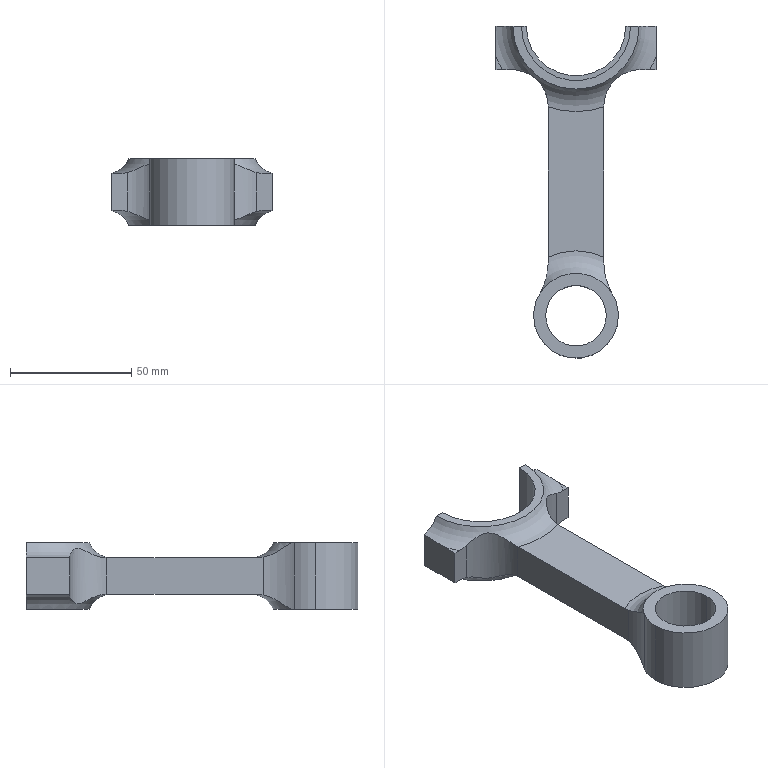Part | SolidWorks | features Fillet 4, ICE 3, Extrusion 1, MirrorPattern 1 | 1 solid | 34 faces | box 66 x 137 x 27.5 mm | volume 56707 mm3 | plane 19 | cylinder 11 | torus 4 | commonest cylinder face diameters 35 x3 25 x2 30 x2 50 x2 41 x1 45 x1
STEP:
#1=CARTESIAN_POINT('',(-12.5,-110.5,13.75));
#2=VERTEX_POINT('',#1);
#3=CARTESIAN_POINT('',(12.5,-110.5,13.75));
#4=VERTEX_POINT('',#3);
#5=CARTESIAN_POINT('',(0.,-110.5,13.75));
#6=DIRECTION('',(0.,0.,1.));
#7=DIRECTION('',(1.,0.,0.));
#8=AXIS2_PLACEMENT_3D('',#5,#6,#7);
#9=CIRCLE('',#8,12.5);
#10=EDGE_CURVE('',#2,#4,#9,.T.);
#11=ORIENTED_EDGE('',*,*,#10,.T.);
#12=CARTESIAN_POINT('',(12.5,-110.5,-13.75));
#13=VERTEX_POINT('',#12);
#14=CARTESIAN_POINT('',(12.5,-110.5,13.75));
#15=DIRECTION('',(0.,0.,-1.));
#16=VECTOR('',#15,1000.);
#17=LINE('',#14,#16);
#18=EDGE_CURVE('',#4,#13,#17,.T.);
#19=ORIENTED_EDGE('',*,*,#18,.T.);
#20=CARTESIAN_POINT('',(-12.5,-110.5,-13.75));
#21=VERTEX_POINT('',#20);
#22=CARTESIAN_POINT('',(0.,-110.5,-13.75));
#23=DIRECTION('',(0.,0.,1.));
#24=DIRECTION('',(1.,0.,0.));
#25=AXIS2_PLACEMENT_3D('',#22,#23,#24);
#26=CIRCLE('',#25,12.5);
#27=EDGE_CURVE('',#21,#13,#26,.T.);
#28=ORIENTED_EDGE('',*,*,#27,.F.);
#29=CARTESIAN_POINT('',(-12.5,-110.5,13.75));
#30=DIRECTION('',(0.,0.,-1.));
#31=VECTOR('',#30,1000.);
#32=LINE('',#29,#31);
#33=EDGE_CURVE('',#2,#21,#32,.T.);
#34=ORIENTED_EDGE('',*,*,#33,.F.);
#35=EDGE_LOOP('',(#11,#19,#28,#34));
#36=FACE_OUTER_BOUND('',#35,.T.);
#37=CARTESIAN_POINT('',(0.,-110.5,13.75));
#38=DIRECTION('',(0.,0.,-1.));
#39=DIRECTION('',(-1.,0.,0.));
#40=AXIS2_PLACEMENT_3D('',#37,#38,#39);
#41=CYLINDRICAL_SURFACE('',#40,12.5);
#42=ADVANCED_FACE('',(#36),#41,.F.);
#43=CARTESIAN_POINT('',(17.5,-110.5,13.75));
#44=VERTEX_POINT('',#43);
#45=CARTESIAN_POINT('',(15.029,-101.535,13.75));
#46=VERTEX_POINT('',#45);
#47=CARTESIAN_POINT('',(0.,-110.5,13.75));
#48=DIRECTION('',(0.,0.,1.));
#49=DIRECTION('',(1.,0.,0.));
#50=AXIS2_PLACEMENT_3D('',#47,#48,#49);
#51=CIRCLE('',#50,17.5);
#52=EDGE_CURVE('',#44,#46,#51,.T.);
#53=ORIENTED_EDGE('',*,*,#52,.F.);
#54=CARTESIAN_POINT('',(17.5,-110.5,-13.75));
#55=VERTEX_POINT('',#54);
#56=CARTESIAN_POINT('',(17.5,-110.5,13.75));
#57=DIRECTION('',(0.,0.,-1.));
#58=VECTOR('',#57,1000.);
#59=LINE('',#56,#58);
#60=EDGE_CURVE('',#44,#55,#59,.T.);
#61=ORIENTED_EDGE('',*,*,#60,.T.);
#62=CARTESIAN_POINT('',(15.029,-101.535,-13.75));
#63=VERTEX_POINT('',#62);
#64=CARTESIAN_POINT('',(0.,-110.5,-13.75));
#65=DIRECTION('',(0.,0.,1.));
#66=DIRECTION('',(1.,0.,0.));
#67=AXIS2_PLACEMENT_3D('',#64,#65,#66);
#68=CIRCLE('',#67,17.5);
#69=EDGE_CURVE('',#55,#63,#68,.T.);
#70=ORIENTED_EDGE('',*,*,#69,.T.);
#71=CARTESIAN_POINT('',(15.029,-101.535,13.75));
#72=DIRECTION('',(0.,0.,1.));
#73=VECTOR('',#72,1000.);
#74=LINE('',#71,#73);
#75=EDGE_CURVE('',#63,#46,#74,.T.);
#76=ORIENTED_EDGE('',*,*,#75,.T.);
#77=EDGE_LOOP('',(#53,#61,#70,#76));
#78=FACE_OUTER_BOUND('',#77,.T.);
#79=CARTESIAN_POINT('',(0.,-110.5,13.75));
#80=DIRECTION('',(0.,0.,-1.));
#81=DIRECTION('',(-1.,0.,0.));
#82=AXIS2_PLACEMENT_3D('',#79,#80,#81);
#83=CYLINDRICAL_SURFACE('',#82,17.5);
#84=ADVANCED_FACE('',(#78),#83,.T.);
#85=ORIENTED_EDGE('',*,*,#60,.F.);
#86=CARTESIAN_POINT('',(-17.5,-110.5,13.75));
#87=VERTEX_POINT('',#86);
#88=CARTESIAN_POINT('',(0.,-110.5,13.75));
#89=DIRECTION('',(0.,0.,1.));
#90=DIRECTION('',(1.,0.,0.));
#91=AXIS2_PLACEMENT_3D('',#88,#89,#90);
#92=CIRCLE('',#91,17.5);
#93=EDGE_CURVE('',#87,#44,#92,.T.);
#94=ORIENTED_EDGE('',*,*,#93,.F.);
#95=CARTESIAN_POINT('',(-17.5,-110.5,-13.75));
#96=VERTEX_POINT('',#95);
#97=CARTESIAN_POINT('',(-17.5,-110.5,13.75));
#98=DIRECTION('',(0.,0.,-1.));
#99=VECTOR('',#98,1000.);
#100=LINE('',#97,#99);
#101=EDGE_CURVE('',#87,#96,#100,.T.);
#102=ORIENTED_EDGE('',*,*,#101,.T.);
#103=CARTESIAN_POINT('',(0.,-110.5,-13.75));
#104=DIRECTION('',(0.,0.,1.));
#105=DIRECTION('',(1.,0.,0.));
#106=AXIS2_PLACEMENT_3D('',#103,#104,#105);
#107=CIRCLE('',#106,17.5);
#108=EDGE_CURVE('',#96,#55,#107,.T.);
#109=ORIENTED_EDGE('',*,*,#108,.T.);
#110=EDGE_LOOP('',(#85,#94,#102,#109));
#111=FACE_OUTER_BOUND('',#110,.T.);
#112=CARTESIAN_POINT('',(0.,-110.5,13.75));
#113=DIRECTION('',(0.,0.,-1.));
#114=DIRECTION('',(-1.,0.,0.));
#115=AXIS2_PLACEMENT_3D('',#112,#113,#114);
#116=CYLINDRICAL_SURFACE('',#115,17.5);
#117=ADVANCED_FACE('',(#111),#116,.T.);
#118=CARTESIAN_POINT('',(26.,9.,-13.75));
#119=VERTEX_POINT('',#118);
#120=CARTESIAN_POINT('',(20.5,9.,-13.75));
#121=VERTEX_POINT('',#120);
#122=CARTESIAN_POINT('',(33.,9.,-13.75));
#123=DIRECTION('',(-1.,0.,0.));
#124=VECTOR('',#123,1000.);
#125=LINE('',#122,#124);
#126=EDGE_CURVE('',#119,#121,#125,.T.);
#127=ORIENTED_EDGE('',*,*,#126,.T.);
#128=CARTESIAN_POINT('',(20.5,9.,-12.75));
#129=VERTEX_POINT('',#128);
#130=CARTESIAN_POINT('',(20.5,9.,-14.97));
#131=DIRECTION('',(0.,0.,1.));
#132=VECTOR('',#131,1000.);
#133=LINE('',#130,#132);
#134=EDGE_CURVE('',#121,#129,#133,.T.);
#135=ORIENTED_EDGE('',*,*,#134,.T.);
#136=CARTESIAN_POINT('',(22.5,9.,-12.75));
#137=VERTEX_POINT('',#136);
#138=CARTESIAN_POINT('',(33.,9.,-12.75));
#139=DIRECTION('',(-1.,0.,0.));
#140=VECTOR('',#139,1000.);
#141=LINE('',#138,#140);
#142=EDGE_CURVE('',#137,#129,#141,.T.);
#143=ORIENTED_EDGE('',*,*,#142,.F.);
#144=CARTESIAN_POINT('',(22.5,9.,13.75));
#145=VERTEX_POINT('',#144);
#146=CARTESIAN_POINT('',(22.5,9.,-12.75));
#147=DIRECTION('',(0.,0.,1.));
#148=VECTOR('',#147,1000.);
#149=LINE('',#146,#148);
#150=EDGE_CURVE('',#137,#145,#149,.T.);
#151=ORIENTED_EDGE('',*,*,#150,.T.);
#152=CARTESIAN_POINT('',(26.,9.,13.75));
#153=VERTEX_POINT('',#152);
#154=CARTESIAN_POINT('',(33.,9.,13.75));
#155=DIRECTION('',(-1.,0.,0.));
#156=VECTOR('',#155,1000.);
#157=LINE('',#154,#156);
#158=EDGE_CURVE('',#153,#145,#157,.T.);
#159=ORIENTED_EDGE('',*,*,#158,.F.);
#160=CARTESIAN_POINT('',(33.,9.,7.761));
#161=VERTEX_POINT('',#160);
#162=CARTESIAN_POINT('',(35.27,9.,17.5));
#163=DIRECTION('',(0.,-1.,0.));
#164=DIRECTION('',(1.,0.,0.));
#165=AXIS2_PLACEMENT_3D('',#162,#163,#164);
#166=CIRCLE('',#165,10.);
#167=EDGE_CURVE('',#153,#161,#166,.T.);
#168=ORIENTED_EDGE('',*,*,#167,.T.);
#169=CARTESIAN_POINT('',(33.,9.,-7.761));
#170=VERTEX_POINT('',#169);
#171=CARTESIAN_POINT('',(33.,9.,13.75));
#172=DIRECTION('',(0.,0.,-1.));
#173=VECTOR('',#172,1000.);
#174=LINE('',#171,#173);
#175=EDGE_CURVE('',#161,#170,#174,.T.);
#176=ORIENTED_EDGE('',*,*,#175,.T.);
#177=CARTESIAN_POINT('',(35.27,9.,-17.5));
#178=DIRECTION('',(0.,-1.,0.));
#179=DIRECTION('',(1.,0.,0.));
#180=AXIS2_PLACEMENT_3D('',#177,#178,#179);
#181=CIRCLE('',#180,10.);
#182=EDGE_CURVE('',#170,#119,#181,.T.);
#183=ORIENTED_EDGE('',*,*,#182,.T.);
#184=EDGE_LOOP('',(#127,#135,#143,#151,#159,#168,#176,#183));
#185=FACE_OUTER_BOUND('',#184,.T.);
#186=CARTESIAN_POINT('',(33.,9.,13.75));
#187=DIRECTION('',(0.,-1.,0.));
#188=DIRECTION('',(1.,0.,0.));
#189=AXIS2_PLACEMENT_3D('',#186,#187,#188);
#190=PLANE('',#189);
#191=ADVANCED_FACE('',(#185),#190,.F.);
#192=CARTESIAN_POINT('',(-33.,-3.45,-7.5));
#193=VERTEX_POINT('',#192);
#194=CARTESIAN_POINT('',(-33.,-9.,-7.5));
#195=VERTEX_POINT('',#194);
#196=CARTESIAN_POINT('',(-33.,0.,-7.5));
#197=DIRECTION('',(0.,-1.,0.));
#198=VECTOR('',#197,1000.);
#199=LINE('',#196,#198);
#200=EDGE_CURVE('',#193,#195,#199,.T.);
#201=ORIENTED_EDGE('',*,*,#200,.F.);
#202=CARTESIAN_POINT('',(-30.331,-9.,-7.5));
#203=VERTEX_POINT('',#202);
#204=CARTESIAN_POINT('',(0.,9.,-7.5));
#205=DIRECTION('',(0.,0.,1.));
#206=DIRECTION('',(-1.,0.,0.));
#207=AXIS2_PLACEMENT_3D('',#204,#205,#206);
#208=CIRCLE('',#207,35.27);
#209=EDGE_CURVE('',#193,#203,#208,.T.);
#210=ORIENTED_EDGE('',*,*,#209,.T.);
#211=CARTESIAN_POINT('',(0.,-9.,-7.5));
#212=DIRECTION('',(1.,0.,0.));
#213=VECTOR('',#212,1000.);
#214=LINE('',#211,#213);
#215=EDGE_CURVE('',#195,#203,#214,.T.);
#216=ORIENTED_EDGE('',*,*,#215,.F.);
#217=EDGE_LOOP('',(#201,#210,#216));
#218=FACE_OUTER_BOUND('',#217,.T.);
#219=CARTESIAN_POINT('',(0.,0.,-7.5));
#220=DIRECTION('',(0.,0.,-1.));
#221=DIRECTION('',(1.,0.,0.));
#222=AXIS2_PLACEMENT_3D('',#219,#220,#221);
#223=PLANE('',#222);
#224=ADVANCED_FACE('',(#218),#223,.T.);
#225=CARTESIAN_POINT('',(11.5,-86.326,-7.5));
#226=VERTEX_POINT('',#225);
#227=CARTESIAN_POINT('',(11.5,-24.343,-7.5));
#228=VERTEX_POINT('',#227);
#229=CARTESIAN_POINT('',(11.5,0.,-7.5));
#230=DIRECTION('',(0.,1.,0.));
#231=VECTOR('',#230,1000.);
#232=LINE('',#229,#231);
#233=EDGE_CURVE('',#226,#228,#232,.T.);
#234=ORIENTED_EDGE('',*,*,#233,.F.);
#235=CARTESIAN_POINT('',(-11.5,-86.326,-7.5));
#236=VERTEX_POINT('',#235);
#237=CARTESIAN_POINT('',(0.,-110.5,-7.5));
#238=DIRECTION('',(0.,0.,1.));
#239=DIRECTION('',(-1.,0.,0.));
#240=AXIS2_PLACEMENT_3D('',#237,#238,#239);
#241=CIRCLE('',#240,26.77);
#242=EDGE_CURVE('',#226,#236,#241,.T.);
#243=ORIENTED_EDGE('',*,*,#242,.T.);
#244=CARTESIAN_POINT('',(-11.5,-24.343,-7.5));
#245=VERTEX_POINT('',#244);
#246=CARTESIAN_POINT('',(-11.5,0.,-7.5));
#247=DIRECTION('',(0.,-1.,0.));
#248=VECTOR('',#247,1000.);
#249=LINE('',#246,#248);
#250=EDGE_CURVE('',#245,#236,#249,.T.);
#251=ORIENTED_EDGE('',*,*,#250,.F.);
#252=CARTESIAN_POINT('',(0.,9.,-7.5));
#253=DIRECTION('',(0.,0.,1.));
#254=DIRECTION('',(-1.,0.,0.));
#255=AXIS2_PLACEMENT_3D('',#252,#253,#254);
#256=CIRCLE('',#255,35.27);
#257=EDGE_CURVE('',#245,#228,#256,.T.);
#258=ORIENTED_EDGE('',*,*,#257,.T.);
#259=EDGE_LOOP('',(#234,#243,#251,#258));
#260=FACE_OUTER_BOUND('',#259,.T.);
#261=CARTESIAN_POINT('',(0.,0.,-7.5));
#262=DIRECTION('',(0.,0.,-1.));
#263=DIRECTION('',(1.,0.,0.));
#264=AXIS2_PLACEMENT_3D('',#261,#262,#263);
#265=PLANE('',#264);
#266=ADVANCED_FACE('',(#260),#265,.T.);
#267=CARTESIAN_POINT('',(33.,-9.,7.5));
#268=VERTEX_POINT('',#267);
#269=CARTESIAN_POINT('',(33.,-3.45,7.5));
#270=VERTEX_POINT('',#269);
#271=CARTESIAN_POINT('',(33.,0.,7.5));
#272=DIRECTION('',(0.,1.,0.));
#273=VECTOR('',#272,1000.);
#274=LINE('',#271,#273);
#275=EDGE_CURVE('',#268,#270,#274,.T.);
#276=ORIENTED_EDGE('',*,*,#275,.T.);
#277=CARTESIAN_POINT('',(30.331,-9.,7.5));
#278=VERTEX_POINT('',#277);
#279=CARTESIAN_POINT('',(0.,9.,7.5));
#280=DIRECTION('',(0.,0.,-1.));
#281=DIRECTION('',(1.,0.,0.));
#282=AXIS2_PLACEMENT_3D('',#279,#280,#281);
#283=CIRCLE('',#282,35.27);
#284=EDGE_CURVE('',#270,#278,#283,.T.);
#285=ORIENTED_EDGE('',*,*,#284,.T.);
#286=CARTESIAN_POINT('',(0.,-9.,7.5));
#287=DIRECTION('',(1.,0.,0.));
#288=VECTOR('',#287,1000.);
#289=LINE('',#286,#288);
#290=EDGE_CURVE('',#278,#268,#289,.T.);
#291=ORIENTED_EDGE('',*,*,#290,.T.);
#292=EDGE_LOOP('',(#276,#285,#291));
#293=FACE_OUTER_BOUND('',#292,.T.);
#294=CARTESIAN_POINT('',(0.,0.,7.5));
#295=DIRECTION('',(0.,0.,1.));
#296=DIRECTION('',(1.,0.,0.));
#297=AXIS2_PLACEMENT_3D('',#294,#295,#296);
#298=PLANE('',#297);
#299=ADVANCED_FACE('',(#293),#298,.T.);
#300=CARTESIAN_POINT('',(-11.5,-24.343,7.5));
#301=VERTEX_POINT('',#300);
#302=CARTESIAN_POINT('',(-11.5,-86.326,7.5));
#303=VERTEX_POINT('',#302);
#304=CARTESIAN_POINT('',(-11.5,0.,7.5));
#305=DIRECTION('',(0.,-1.,0.));
#306=VECTOR('',#305,1000.);
#307=LINE('',#304,#306);
#308=EDGE_CURVE('',#301,#303,#307,.T.);
#309=ORIENTED_EDGE('',*,*,#308,.T.);
#310=CARTESIAN_POINT('',(11.5,-86.326,7.5));
#311=VERTEX_POINT('',#310);
#312=CARTESIAN_POINT('',(0.,-110.5,7.5));
#313=DIRECTION('',(0.,0.,-1.));
#314=DIRECTION('',(1.,0.,0.));
#315=AXIS2_PLACEMENT_3D('',#312,#313,#314);
#316=CIRCLE('',#315,26.77);
#317=EDGE_CURVE('',#303,#311,#316,.T.);
#318=ORIENTED_EDGE('',*,*,#317,.T.);
#319=CARTESIAN_POINT('',(11.5,-24.343,7.5));
#320=VERTEX_POINT('',#319);
#321=CARTESIAN_POINT('',(11.5,0.,7.5));
#322=DIRECTION('',(0.,1.,0.));
#323=VECTOR('',#322,1000.);
#324=LINE('',#321,#323);
#325=EDGE_CURVE('',#311,#320,#324,.T.);
#326=ORIENTED_EDGE('',*,*,#325,.T.);
#327=CARTESIAN_POINT('',(0.,9.,7.5));
#328=DIRECTION('',(0.,0.,-1.));
#329=DIRECTION('',(1.,0.,0.));
#330=AXIS2_PLACEMENT_3D('',#327,#328,#329);
#331=CIRCLE('',#330,35.27);
#332=EDGE_CURVE('',#320,#301,#331,.T.);
#333=ORIENTED_EDGE('',*,*,#332,.T.);
#334=EDGE_LOOP('',(#309,#318,#326,#333));
#335=FACE_OUTER_BOUND('',#334,.T.);
#336=CARTESIAN_POINT('',(0.,0.,7.5));
#337=DIRECTION('',(0.,0.,1.));
#338=DIRECTION('',(1.,0.,0.));
#339=AXIS2_PLACEMENT_3D('',#336,#337,#338);
#340=PLANE('',#339);
#341=ADVANCED_FACE('',(#335),#340,.T.);
#342=CARTESIAN_POINT('',(-33.,9.,7.761));
#343=VERTEX_POINT('',#342);
#344=CARTESIAN_POINT('',(-33.,9.,-7.761));
#345=VERTEX_POINT('',#344);
#346=CARTESIAN_POINT('',(-33.,9.,13.75));
#347=DIRECTION('',(0.,0.,-1.));
#348=VECTOR('',#347,1000.);
#349=LINE('',#346,#348);
#350=EDGE_CURVE('',#343,#345,#349,.T.);
#351=ORIENTED_EDGE('',*,*,#350,.T.);
#352=CARTESIAN_POINT('',(-33.,9.,-7.761));
#353=CARTESIAN_POINT('',(-33.,7.962,-7.761));
#354=CARTESIAN_POINT('',(-33.,6.925,-7.749));
#355=CARTESIAN_POINT('',(-33.,4.85,-7.707));
#356=CARTESIAN_POINT('',(-33.,3.812,-7.676));
#357=CARTESIAN_POINT('',(-33.,0.7007,-7.578));
#358=CARTESIAN_POINT('',(-33.,-1.373,-7.5));
#359=CARTESIAN_POINT('',(-33.,-3.45,-7.5));
#360=B_SPLINE_CURVE_WITH_KNOTS('',3,(#352,#353,#354,#355,#356,#357,#358,#359),.UNSPECIFIED.,.F.,.F.,(4,2,2,4),(0.,0.003113,0.006226,0.01245),.UNSPECIFIED.);
#361=EDGE_CURVE('',#345,#193,#360,.T.);
#362=ORIENTED_EDGE('',*,*,#361,.T.);
#363=ORIENTED_EDGE('',*,*,#200,.T.);
#364=CARTESIAN_POINT('',(-33.,-9.,7.5));
#365=VERTEX_POINT('',#364);
#366=CARTESIAN_POINT('',(-33.,-9.,13.75));
#367=DIRECTION('',(0.,0.,-1.));
#368=VECTOR('',#367,1000.);
#369=LINE('',#366,#368);
#370=EDGE_CURVE('',#365,#195,#369,.T.);
#371=ORIENTED_EDGE('',*,*,#370,.F.);
#372=CARTESIAN_POINT('',(-33.,-3.45,7.5));
#373=VERTEX_POINT('',#372);
#374=CARTESIAN_POINT('',(-33.,0.,7.5));
#375=DIRECTION('',(0.,-1.,0.));
#376=VECTOR('',#375,1000.);
#377=LINE('',#374,#376);
#378=EDGE_CURVE('',#373,#365,#377,.T.);
#379=ORIENTED_EDGE('',*,*,#378,.F.);
#380=CARTESIAN_POINT('',(-33.,-3.45,7.5));
#381=CARTESIAN_POINT('',(-33.,-1.374,7.5));
#382=CARTESIAN_POINT('',(-33.,0.7005,7.578));
#383=CARTESIAN_POINT('',(-33.,3.812,7.676));
#384=CARTESIAN_POINT('',(-33.,4.849,7.707));
#385=CARTESIAN_POINT('',(-33.,6.924,7.749));
#386=CARTESIAN_POINT('',(-33.,7.962,7.761));
#387=CARTESIAN_POINT('',(-33.,9.,7.761));
#388=B_SPLINE_CURVE_WITH_KNOTS('',3,(#380,#381,#382,#383,#384,#385,#386,#387),.UNSPECIFIED.,.F.,.F.,(4,2,2,4),(0.,0.006226,0.009339,0.01245),.UNSPECIFIED.);
#389=EDGE_CURVE('',#373,#343,#388,.T.);
#390=ORIENTED_EDGE('',*,*,#389,.T.);
#391=EDGE_LOOP('',(#351,#362,#363,#371,#379,#390));
#392=FACE_OUTER_BOUND('',#391,.T.);
#393=CARTESIAN_POINT('',(-33.,-9.,13.75));
#394=DIRECTION('',(1.,0.,0.));
#395=DIRECTION('',(0.,0.,-1.));
#396=AXIS2_PLACEMENT_3D('',#393,#394,#395);
#397=PLANE('',#396);
#398=ADVANCED_FACE('',(#392),#397,.F.);
#399=ORIENTED_EDGE('',*,*,#215,.T.);
#400=CARTESIAN_POINT('',(-26.5,-9.,-8.038));
#401=VERTEX_POINT('',#400);
#402=CARTESIAN_POINT('',(-30.331,-9.,-7.5));
#403=CARTESIAN_POINT('',(-29.029,-9.,-7.5));
#404=CARTESIAN_POINT('',(-27.753,-9.,-7.684));
#405=CARTESIAN_POINT('',(-26.5,-9.,-8.038));
#406=B_SPLINE_CURVE_WITH_KNOTS('',3,(#402,#403,#404,#405),.UNSPECIFIED.,.F.,.F.,(4,4),(0.,0.003869),.UNSPECIFIED.);
#407=EDGE_CURVE('',#203,#401,#406,.T.);
#408=ORIENTED_EDGE('',*,*,#407,.T.);
#409=CARTESIAN_POINT('',(-26.5,-9.,8.038));
#410=VERTEX_POINT('',#409);
#411=CARTESIAN_POINT('',(-26.5,-9.,13.75));
#412=DIRECTION('',(0.,0.,1.));
#413=VECTOR('',#412,1000.);
#414=LINE('',#411,#413);
#415=EDGE_CURVE('',#401,#410,#414,.T.);
#416=ORIENTED_EDGE('',*,*,#415,.T.);
#417=CARTESIAN_POINT('',(-30.331,-9.,7.5));
#418=VERTEX_POINT('',#417);
#419=CARTESIAN_POINT('',(-26.5,-9.,8.038));
#420=CARTESIAN_POINT('',(-27.753,-9.,7.684));
#421=CARTESIAN_POINT('',(-29.029,-9.,7.5));
#422=CARTESIAN_POINT('',(-30.331,-9.,7.5));
#423=B_SPLINE_CURVE_WITH_KNOTS('',3,(#419,#420,#421,#422),.UNSPECIFIED.,.F.,.F.,(4,4),(0.,0.003869),.UNSPECIFIED.);
#424=EDGE_CURVE('',#410,#418,#423,.T.);
#425=ORIENTED_EDGE('',*,*,#424,.T.);
#426=CARTESIAN_POINT('',(0.,-9.,7.5));
#427=DIRECTION('',(1.,0.,0.));
#428=VECTOR('',#427,1000.);
#429=LINE('',#426,#428);
#430=EDGE_CURVE('',#365,#418,#429,.T.);
#431=ORIENTED_EDGE('',*,*,#430,.F.);
#432=ORIENTED_EDGE('',*,*,#370,.T.);
#433=EDGE_LOOP('',(#399,#408,#416,#425,#431,#432));
#434=FACE_OUTER_BOUND('',#433,.T.);
#435=CARTESIAN_POINT('',(-11.5,-9.,13.75));
#436=DIRECTION('',(0.,1.,0.));
#437=DIRECTION('',(-1.,0.,0.));
#438=AXIS2_PLACEMENT_3D('',#435,#436,#437);
#439=PLANE('',#438);
#440=ADVANCED_FACE('',(#434),#439,.F.);
#441=CARTESIAN_POINT('',(-11.5,-24.,7.505));
#442=VERTEX_POINT('',#441);
#443=CARTESIAN_POINT('',(-11.5,-24.,-7.505));
#444=VERTEX_POINT('',#443);
#445=CARTESIAN_POINT('',(-11.5,-24.,-13.75));
#446=DIRECTION('',(0.,0.,-1.));
#447=VECTOR('',#446,1000.);
#448=LINE('',#445,#447);
#449=EDGE_CURVE('',#442,#444,#448,.T.);
#450=ORIENTED_EDGE('',*,*,#449,.T.);
#451=CARTESIAN_POINT('',(-11.5,-24.,-7.505));
#452=CARTESIAN_POINT('',(-11.5,-24.114,-7.502));
#453=CARTESIAN_POINT('',(-11.5,-24.229,-7.5));
#454=CARTESIAN_POINT('',(-11.5,-24.343,-7.5));
#455=B_SPLINE_CURVE_WITH_KNOTS('',3,(#451,#452,#453,#454),.UNSPECIFIED.,.F.,.F.,(4,4),(0.,0.0003428),.UNSPECIFIED.);
#456=EDGE_CURVE('',#444,#245,#455,.T.);
#457=ORIENTED_EDGE('',*,*,#456,.T.);
#458=ORIENTED_EDGE('',*,*,#250,.T.);
#459=CARTESIAN_POINT('',(-11.5,-88.728,-7.733));
#460=VERTEX_POINT('',#459);
#461=CARTESIAN_POINT('',(-11.5,-86.326,-7.5));
#462=CARTESIAN_POINT('',(-11.5,-87.134,-7.5));
#463=CARTESIAN_POINT('',(-11.5,-87.935,-7.579));
#464=CARTESIAN_POINT('',(-11.5,-88.728,-7.733));
#465=B_SPLINE_CURVE_WITH_KNOTS('',3,(#461,#462,#463,#464),.UNSPECIFIED.,.F.,.F.,(4,4),(0.,0.002414),.UNSPECIFIED.);
#466=EDGE_CURVE('',#236,#460,#465,.T.);
#467=ORIENTED_EDGE('',*,*,#466,.T.);
#468=CARTESIAN_POINT('',(-11.5,-88.728,7.733));
#469=VERTEX_POINT('',#468);
#470=CARTESIAN_POINT('',(-11.5,-88.728,13.75));
#471=DIRECTION('',(0.,0.,1.));
#472=VECTOR('',#471,1000.);
#473=LINE('',#470,#472);
#474=EDGE_CURVE('',#460,#469,#473,.T.);
#475=ORIENTED_EDGE('',*,*,#474,.T.);
#476=CARTESIAN_POINT('',(-11.5,-88.728,7.733));
#477=CARTESIAN_POINT('',(-11.5,-87.935,7.579));
#478=CARTESIAN_POINT('',(-11.5,-87.134,7.5));
#479=CARTESIAN_POINT('',(-11.5,-86.326,7.5));
#480=B_SPLINE_CURVE_WITH_KNOTS('',3,(#476,#477,#478,#479),.UNSPECIFIED.,.F.,.F.,(4,4),(0.,0.002414),.UNSPECIFIED.);
#481=EDGE_CURVE('',#469,#303,#480,.T.);
#482=ORIENTED_EDGE('',*,*,#481,.T.);
#483=ORIENTED_EDGE('',*,*,#308,.F.);
#484=CARTESIAN_POINT('',(-11.5,-24.343,7.5));
#485=CARTESIAN_POINT('',(-11.5,-24.229,7.5));
#486=CARTESIAN_POINT('',(-11.5,-24.114,7.502));
#487=CARTESIAN_POINT('',(-11.5,-24.,7.505));
#488=B_SPLINE_CURVE_WITH_KNOTS('',3,(#484,#485,#486,#487),.UNSPECIFIED.,.F.,.F.,(4,4),(0.,0.0003428),.UNSPECIFIED.);
#489=EDGE_CURVE('',#301,#442,#488,.T.);
#490=ORIENTED_EDGE('',*,*,#489,.T.);
#491=EDGE_LOOP('',(#450,#457,#458,#467,#475,#482,#483,#490));
#492=FACE_OUTER_BOUND('',#491,.T.);
#493=CARTESIAN_POINT('',(-11.5,-9.,13.75));
#494=DIRECTION('',(1.,0.,0.));
#495=DIRECTION('',(0.,1.,0.));
#496=AXIS2_PLACEMENT_3D('',#493,#494,#495);
#497=PLANE('',#496);
#498=ADVANCED_FACE('',(#492),#497,.F.);
#499=CARTESIAN_POINT('',(11.5,-88.728,7.733));
#500=VERTEX_POINT('',#499);
#501=CARTESIAN_POINT('',(11.5,-88.728,-7.733));
#502=VERTEX_POINT('',#501);
#503=CARTESIAN_POINT('',(11.5,-88.728,-13.75));
#504=DIRECTION('',(0.,0.,-1.));
#505=VECTOR('',#504,1000.);
#506=LINE('',#503,#505);
#507=EDGE_CURVE('',#500,#502,#506,.T.);
#508=ORIENTED_EDGE('',*,*,#507,.T.);
#509=CARTESIAN_POINT('',(11.5,-88.728,-7.733));
#510=CARTESIAN_POINT('',(11.5,-87.935,-7.579));
#511=CARTESIAN_POINT('',(11.5,-87.134,-7.5));
#512=CARTESIAN_POINT('',(11.5,-86.326,-7.5));
#513=B_SPLINE_CURVE_WITH_KNOTS('',3,(#509,#510,#511,#512),.UNSPECIFIED.,.F.,.F.,(4,4),(0.,0.002414),.UNSPECIFIED.);
#514=EDGE_CURVE('',#502,#226,#513,.T.);
#515=ORIENTED_EDGE('',*,*,#514,.T.);
#516=ORIENTED_EDGE('',*,*,#233,.T.);
#517=CARTESIAN_POINT('',(11.5,-24.,-7.505));
#518=VERTEX_POINT('',#517);
#519=CARTESIAN_POINT('',(11.5,-24.343,-7.5));
#520=CARTESIAN_POINT('',(11.5,-24.229,-7.5));
#521=CARTESIAN_POINT('',(11.5,-24.114,-7.502));
#522=CARTESIAN_POINT('',(11.5,-24.,-7.505));
#523=B_SPLINE_CURVE_WITH_KNOTS('',3,(#519,#520,#521,#522),.UNSPECIFIED.,.F.,.F.,(4,4),(0.,0.0003428),.UNSPECIFIED.);
#524=EDGE_CURVE('',#228,#518,#523,.T.);
#525=ORIENTED_EDGE('',*,*,#524,.T.);
#526=CARTESIAN_POINT('',(11.5,-24.,7.505));
#527=VERTEX_POINT('',#526);
#528=CARTESIAN_POINT('',(11.5,-24.,13.75));
#529=DIRECTION('',(0.,0.,1.));
#530=VECTOR('',#529,1000.);
#531=LINE('',#528,#530);
#532=EDGE_CURVE('',#518,#527,#531,.T.);
#533=ORIENTED_EDGE('',*,*,#532,.T.);
#534=CARTESIAN_POINT('',(11.5,-24.,7.505));
#535=CARTESIAN_POINT('',(11.5,-24.114,7.502));
#536=CARTESIAN_POINT('',(11.5,-24.229,7.5));
#537=CARTESIAN_POINT('',(11.5,-24.343,7.5));
#538=B_SPLINE_CURVE_WITH_KNOTS('',3,(#534,#535,#536,#537),.UNSPECIFIED.,.F.,.F.,(4,4),(0.,0.0003428),.UNSPECIFIED.);
#539=EDGE_CURVE('',#527,#320,#538,.T.);
#540=ORIENTED_EDGE('',*,*,#539,.T.);
#541=ORIENTED_EDGE('',*,*,#325,.F.);
#542=CARTESIAN_POINT('',(11.5,-86.326,7.5));
#543=CARTESIAN_POINT('',(11.5,-87.134,7.5));
#544=CARTESIAN_POINT('',(11.5,-87.935,7.579));
#545=CARTESIAN_POINT('',(11.5,-88.728,7.733));
#546=B_SPLINE_CURVE_WITH_KNOTS('',3,(#542,#543,#544,#545),.UNSPECIFIED.,.F.,.F.,(4,4),(0.,0.002414),.UNSPECIFIED.);
#547=EDGE_CURVE('',#311,#500,#546,.T.);
#548=ORIENTED_EDGE('',*,*,#547,.T.);
#549=EDGE_LOOP('',(#508,#515,#516,#525,#533,#540,#541,#548));
#550=FACE_OUTER_BOUND('',#549,.T.);
#551=CARTESIAN_POINT('',(11.5,-9.,13.75));
#552=DIRECTION('',(-1.,0.,0.));
#553=DIRECTION('',(0.,-1.,0.));
#554=AXIS2_PLACEMENT_3D('',#551,#552,#553);
#555=PLANE('',#554);
#556=ADVANCED_FACE('',(#550),#555,.F.);
#557=CARTESIAN_POINT('',(26.5,-9.,8.038));
#558=VERTEX_POINT('',#557);
#559=CARTESIAN_POINT('',(26.5,-9.,-8.038));
#560=VERTEX_POINT('',#559);
#561=CARTESIAN_POINT('',(26.5,-9.,-13.75));
#562=DIRECTION('',(0.,0.,-1.));
#563=VECTOR('',#562,1000.);
#564=LINE('',#561,#563);
#565=EDGE_CURVE('',#558,#560,#564,.T.);
#566=ORIENTED_EDGE('',*,*,#565,.T.);
#567=CARTESIAN_POINT('',(30.331,-9.,-7.5));
#568=VERTEX_POINT('',#567);
#569=CARTESIAN_POINT('',(26.5,-9.,-8.038));
#570=CARTESIAN_POINT('',(27.753,-9.,-7.684));
#571=CARTESIAN_POINT('',(29.029,-9.,-7.5));
#572=CARTESIAN_POINT('',(30.331,-9.,-7.5));
#573=B_SPLINE_CURVE_WITH_KNOTS('',3,(#569,#570,#571,#572),.UNSPECIFIED.,.F.,.F.,(4,4),(0.,0.003869),.UNSPECIFIED.);
#574=EDGE_CURVE('',#560,#568,#573,.T.);
#575=ORIENTED_EDGE('',*,*,#574,.T.);
#576=CARTESIAN_POINT('',(33.,-9.,-7.5));
#577=VERTEX_POINT('',#576);
#578=CARTESIAN_POINT('',(0.,-9.,-7.5));
#579=DIRECTION('',(1.,0.,0.));
#580=VECTOR('',#579,1000.);
#581=LINE('',#578,#580);
#582=EDGE_CURVE('',#568,#577,#581,.T.);
#583=ORIENTED_EDGE('',*,*,#582,.T.);
#584=CARTESIAN_POINT('',(33.,-9.,13.75));
#585=DIRECTION('',(0.,0.,-1.));
#586=VECTOR('',#585,1000.);
#587=LINE('',#584,#586);
#588=EDGE_CURVE('',#268,#577,#587,.T.);
#589=ORIENTED_EDGE('',*,*,#588,.F.);
#590=ORIENTED_EDGE('',*,*,#290,.F.);
#591=CARTESIAN_POINT('',(30.331,-9.,7.5));
#592=CARTESIAN_POINT('',(29.029,-9.,7.5));
#593=CARTESIAN_POINT('',(27.753,-9.,7.684));
#594=CARTESIAN_POINT('',(26.5,-9.,8.038));
#595=B_SPLINE_CURVE_WITH_KNOTS('',3,(#591,#592,#593,#594),.UNSPECIFIED.,.F.,.F.,(4,4),(0.,0.003869),.UNSPECIFIED.);
#596=EDGE_CURVE('',#278,#558,#595,.T.);
#597=ORIENTED_EDGE('',*,*,#596,.T.);
#598=EDGE_LOOP('',(#566,#575,#583,#589,#590,#597));
#599=FACE_OUTER_BOUND('',#598,.T.);
#600=CARTESIAN_POINT('',(33.,-9.,13.75));
#601=DIRECTION('',(0.,1.,0.));
#602=DIRECTION('',(-1.,0.,0.));
#603=AXIS2_PLACEMENT_3D('',#600,#601,#602);
#604=PLANE('',#603);
#605=ADVANCED_FACE('',(#599),#604,.F.);
#606=CARTESIAN_POINT('',(33.,-3.45,-7.5));
#607=VERTEX_POINT('',#606);
#608=CARTESIAN_POINT('',(33.,0.,-7.5));
#609=DIRECTION('',(0.,1.,0.));
#610=VECTOR('',#609,1000.);
#611=LINE('',#608,#610);
#612=EDGE_CURVE('',#577,#607,#611,.T.);
#613=ORIENTED_EDGE('',*,*,#612,.T.);
#614=CARTESIAN_POINT('',(33.,-3.45,-7.5));
#615=CARTESIAN_POINT('',(33.,-1.374,-7.5));
#616=CARTESIAN_POINT('',(33.,0.7005,-7.578));
#617=CARTESIAN_POINT('',(33.,3.812,-7.676));
#618=CARTESIAN_POINT('',(33.,4.849,-7.707));
#619=CARTESIAN_POINT('',(33.,6.924,-7.749));
#620=CARTESIAN_POINT('',(33.,7.962,-7.761));
#621=CARTESIAN_POINT('',(33.,9.,-7.761));
#622=B_SPLINE_CURVE_WITH_KNOTS('',3,(#614,#615,#616,#617,#618,#619,#620,#621),.UNSPECIFIED.,.F.,.F.,(4,2,2,4),(0.,0.006226,0.009339,0.01245),.UNSPECIFIED.);
#623=EDGE_CURVE('',#607,#170,#622,.T.);
#624=ORIENTED_EDGE('',*,*,#623,.T.);
#625=ORIENTED_EDGE('',*,*,#175,.F.);
#626=CARTESIAN_POINT('',(33.,9.,7.761));
#627=CARTESIAN_POINT('',(33.,7.962,7.761));
#628=CARTESIAN_POINT('',(33.,6.925,7.749));
#629=CARTESIAN_POINT('',(33.,4.85,7.707));
#630=CARTESIAN_POINT('',(33.,3.812,7.676));
#631=CARTESIAN_POINT('',(33.,0.7007,7.578));
#632=CARTESIAN_POINT('',(33.,-1.373,7.5));
#633=CARTESIAN_POINT('',(33.,-3.45,7.5));
#634=B_SPLINE_CURVE_WITH_KNOTS('',3,(#626,#627,#628,#629,#630,#631,#632,#633),.UNSPECIFIED.,.F.,.F.,(4,2,2,4),(0.,0.003113,0.006226,0.01245),.UNSPECIFIED.);
#635=EDGE_CURVE('',#161,#270,#634,.T.);
#636=ORIENTED_EDGE('',*,*,#635,.T.);
#637=ORIENTED_EDGE('',*,*,#275,.F.);
#638=ORIENTED_EDGE('',*,*,#588,.T.);
#639=EDGE_LOOP('',(#613,#624,#625,#636,#637,#638));
#640=FACE_OUTER_BOUND('',#639,.T.);
#641=CARTESIAN_POINT('',(33.,-9.,13.75));
#642=DIRECTION('',(-1.,0.,0.));
#643=DIRECTION('',(0.,0.,1.));
#644=AXIS2_PLACEMENT_3D('',#641,#642,#643);
#645=PLANE('',#644);
#646=ADVANCED_FACE('',(#640),#645,.F.);
#647=ORIENTED_EDGE('',*,*,#415,.F.);
#648=CARTESIAN_POINT('',(-26.5,-9.,-8.038));
#649=CARTESIAN_POINT('',(-25.495,-9.,-8.322));
#650=CARTESIAN_POINT('',(-24.539,-9.099,-8.689));
#651=CARTESIAN_POINT('',(-23.144,-9.372,-9.291));
#652=CARTESIAN_POINT('',(-22.686,-9.485,-9.5));
#653=CARTESIAN_POINT('',(-21.779,-9.755,-9.921));
#654=CARTESIAN_POINT('',(-21.329,-9.911,-10.132));
#655=CARTESIAN_POINT('',(-20.445,-10.268,-10.533));
#656=CARTESIAN_POINT('',(-20.009,-10.468,-10.723));
#657=CARTESIAN_POINT('',(-19.358,-10.807,-10.971));
#658=CARTESIAN_POINT('',(-19.141,-10.927,-11.048));
#659=CARTESIAN_POINT('',(-18.707,-11.181,-11.184));
#660=CARTESIAN_POINT('',(-18.49,-11.315,-11.244));
#661=CARTESIAN_POINT('',(-17.852,-11.734,-11.387));
#662=CARTESIAN_POINT('',(-17.437,-12.036,-11.436));
#663=CARTESIAN_POINT('',(-16.832,-12.529,-11.426));
#664=CARTESIAN_POINT('',(-16.633,-12.699,-11.409));
#665=CARTESIAN_POINT('',(-16.25,-13.045,-11.349));
#666=CARTESIAN_POINT('',(-16.065,-13.221,-11.306));
#667=CARTESIAN_POINT('',(-15.529,-13.758,-11.146));
#668=CARTESIAN_POINT('',(-15.193,-14.131,-10.996));
#669=CARTESIAN_POINT('',(-14.573,-14.89,-10.651));
#670=CARTESIAN_POINT('',(-14.289,-15.275,-10.457));
#671=CARTESIAN_POINT('',(-13.763,-16.063,-10.052));
#672=CARTESIAN_POINT('',(-13.52,-16.467,-9.842));
#673=CARTESIAN_POINT('',(-13.073,-17.297,-9.423));
#674=CARTESIAN_POINT('',(-12.867,-17.726,-9.213));
#675=CARTESIAN_POINT('',(-12.308,-19.05,-8.613));
#676=CARTESIAN_POINT('',(-12.017,-19.971,-8.255));
#677=CARTESIAN_POINT('',(-11.712,-21.436,-7.85));
#678=CARTESIAN_POINT('',(-11.633,-21.942,-7.737));
#679=CARTESIAN_POINT('',(-11.527,-22.962,-7.573));
#680=CARTESIAN_POINT('',(-11.5,-23.478,-7.521));
#681=CARTESIAN_POINT('',(-11.5,-24.,-7.505));
#682=B_SPLINE_CURVE_WITH_KNOTS('',3,(#648,#649,#650,#651,#652,#653,#654,#655,#656,#657,#658,#659,#660,#661,#662,#663,#664,#665,#666,#667,#668,#669,#670,#671,#672,#673,#674,#675,#676,#677,#678,#679,#680,#681),.UNSPECIFIED.,.F.,.F.,(4,2,2,2,2,2,2,2,2,2,2,2,2,2,2,2,4),(0.,0.003083,0.004625,0.006166,0.007708,0.008479,0.009249,0.01079,0.01156,0.01233,0.01387,0.01542,0.01696,0.0185,0.02158,0.02312,0.02467),.UNSPECIFIED.);
#683=EDGE_CURVE('',#401,#444,#682,.T.);
#684=ORIENTED_EDGE('',*,*,#683,.T.);
#685=ORIENTED_EDGE('',*,*,#449,.F.);
#686=CARTESIAN_POINT('',(-11.5,-24.,7.505));
#687=CARTESIAN_POINT('',(-11.5,-22.953,7.537));
#688=CARTESIAN_POINT('',(-11.608,-21.944,7.711));
#689=CARTESIAN_POINT('',(-11.912,-20.475,8.115));
#690=CARTESIAN_POINT('',(-12.037,-19.991,8.275));
#691=CARTESIAN_POINT('',(-12.328,-19.062,8.623));
#692=CARTESIAN_POINT('',(-12.493,-18.612,8.812));
#693=CARTESIAN_POINT('',(-12.862,-17.737,9.208));
#694=CARTESIAN_POINT('',(-13.065,-17.312,9.416));
#695=CARTESIAN_POINT('',(-13.512,-16.48,9.835));
#696=CARTESIAN_POINT('',(-13.757,-16.073,10.048));
#697=CARTESIAN_POINT('',(-14.286,-15.279,10.455));
#698=CARTESIAN_POINT('',(-14.571,-14.893,10.649));
#699=CARTESIAN_POINT('',(-15.033,-14.327,10.907));
#700=CARTESIAN_POINT('',(-15.193,-14.14,10.987));
#701=CARTESIAN_POINT('',(-15.527,-13.77,11.132));
#702=CARTESIAN_POINT('',(-15.701,-13.586,11.197));
#703=CARTESIAN_POINT('',(-16.24,-13.046,11.358));
#704=CARTESIAN_POINT('',(-16.619,-12.702,11.421));
#705=CARTESIAN_POINT('',(-17.221,-12.211,11.433));
#706=CARTESIAN_POINT('',(-17.429,-12.051,11.423));
#707=CARTESIAN_POINT('',(-17.847,-11.744,11.377));
#708=CARTESIAN_POINT('',(-18.058,-11.598,11.341));
#709=CARTESIAN_POINT('',(-18.696,-11.18,11.198));
#710=CARTESIAN_POINT('',(-19.129,-10.927,11.058));
#711=CARTESIAN_POINT('',(-20.003,-10.471,10.726));
#712=CARTESIAN_POINT('',(-20.44,-10.27,10.536));
#713=CARTESIAN_POINT('',(-21.762,-9.736,9.937));
#714=CARTESIAN_POINT('',(-22.658,-9.469,9.501));
#715=CARTESIAN_POINT('',(-24.537,-9.098,8.69));
#716=CARTESIAN_POINT('',(-25.498,-9.,8.321));
#717=CARTESIAN_POINT('',(-26.5,-9.,8.038));
#718=B_SPLINE_CURVE_WITH_KNOTS('',3,(#686,#687,#688,#689,#690,#691,#692,#693,#694,#695,#696,#697,#698,#699,#700,#701,#702,#703,#704,#705,#706,#707,#708,#709,#710,#711,#712,#713,#714,#715,#716,#717),.UNSPECIFIED.,.F.,.F.,(4,2,2,2,2,2,2,2,2,2,2,2,2,2,2,4),(0.,0.003087,0.00463,0.006173,0.007716,0.00926,0.0108,0.01157,0.01235,0.01389,0.01466,0.01543,0.01698,0.01852,0.02161,0.02469),.UNSPECIFIED.);
#719=EDGE_CURVE('',#442,#410,#718,.T.);
#720=ORIENTED_EDGE('',*,*,#719,.T.);
#721=EDGE_LOOP('',(#647,#684,#685,#720));
#722=FACE_OUTER_BOUND('',#721,.T.);
#723=CARTESIAN_POINT('',(-26.5,-24.,13.75));
#724=DIRECTION('',(0.,0.,1.));
#725=DIRECTION('',(1.,0.,0.));
#726=AXIS2_PLACEMENT_3D('',#723,#724,#725);
#727=CYLINDRICAL_SURFACE('',#726,15.);
#728=ADVANCED_FACE('',(#722),#727,.F.);
#729=ORIENTED_EDGE('',*,*,#532,.F.);
#730=CARTESIAN_POINT('',(11.5,-24.,-7.505));
#731=CARTESIAN_POINT('',(11.5,-22.953,-7.537));
#732=CARTESIAN_POINT('',(11.608,-21.944,-7.711));
#733=CARTESIAN_POINT('',(11.912,-20.475,-8.115));
#734=CARTESIAN_POINT('',(12.037,-19.991,-8.275));
#735=CARTESIAN_POINT('',(12.328,-19.062,-8.623));
#736=CARTESIAN_POINT('',(12.493,-18.612,-8.812));
#737=CARTESIAN_POINT('',(12.862,-17.737,-9.208));
#738=CARTESIAN_POINT('',(13.065,-17.312,-9.416));
#739=CARTESIAN_POINT('',(13.512,-16.48,-9.835));
#740=CARTESIAN_POINT('',(13.757,-16.073,-10.048));
#741=CARTESIAN_POINT('',(14.286,-15.279,-10.455));
#742=CARTESIAN_POINT('',(14.571,-14.893,-10.649));
#743=CARTESIAN_POINT('',(15.033,-14.327,-10.907));
#744=CARTESIAN_POINT('',(15.193,-14.14,-10.987));
#745=CARTESIAN_POINT('',(15.527,-13.77,-11.132));
#746=CARTESIAN_POINT('',(15.701,-13.586,-11.197));
#747=CARTESIAN_POINT('',(16.24,-13.046,-11.358));
#748=CARTESIAN_POINT('',(16.619,-12.702,-11.421));
#749=CARTESIAN_POINT('',(17.221,-12.211,-11.433));
#750=CARTESIAN_POINT('',(17.429,-12.051,-11.423));
#751=CARTESIAN_POINT('',(17.847,-11.744,-11.377));
#752=CARTESIAN_POINT('',(18.058,-11.598,-11.341));
#753=CARTESIAN_POINT('',(18.696,-11.18,-11.198));
#754=CARTESIAN_POINT('',(19.129,-10.927,-11.058));
#755=CARTESIAN_POINT('',(20.003,-10.471,-10.726));
#756=CARTESIAN_POINT('',(20.44,-10.27,-10.536));
#757=CARTESIAN_POINT('',(21.762,-9.736,-9.937));
#758=CARTESIAN_POINT('',(22.658,-9.469,-9.501));
#759=CARTESIAN_POINT('',(24.537,-9.098,-8.69));
#760=CARTESIAN_POINT('',(25.498,-9.,-8.321));
#761=CARTESIAN_POINT('',(26.5,-9.,-8.038));
#762=B_SPLINE_CURVE_WITH_KNOTS('',3,(#730,#731,#732,#733,#734,#735,#736,#737,#738,#739,#740,#741,#742,#743,#744,#745,#746,#747,#748,#749,#750,#751,#752,#753,#754,#755,#756,#757,#758,#759,#760,#761),.UNSPECIFIED.,.F.,.F.,(4,2,2,2,2,2,2,2,2,2,2,2,2,2,2,4),(0.,0.003087,0.00463,0.006173,0.007716,0.00926,0.0108,0.01157,0.01235,0.01389,0.01466,0.01543,0.01698,0.01852,0.02161,0.02469),.UNSPECIFIED.);
#763=EDGE_CURVE('',#518,#560,#762,.T.);
#764=ORIENTED_EDGE('',*,*,#763,.T.);
#765=ORIENTED_EDGE('',*,*,#565,.F.);
#766=CARTESIAN_POINT('',(26.5,-9.,8.038));
#767=CARTESIAN_POINT('',(25.495,-9.,8.322));
#768=CARTESIAN_POINT('',(24.539,-9.099,8.689));
#769=CARTESIAN_POINT('',(23.144,-9.372,9.291));
#770=CARTESIAN_POINT('',(22.686,-9.485,9.5));
#771=CARTESIAN_POINT('',(21.779,-9.755,9.921));
#772=CARTESIAN_POINT('',(21.329,-9.911,10.132));
#773=CARTESIAN_POINT('',(20.445,-10.268,10.533));
#774=CARTESIAN_POINT('',(20.009,-10.468,10.723));
#775=CARTESIAN_POINT('',(19.358,-10.807,10.971));
#776=CARTESIAN_POINT('',(19.141,-10.927,11.048));
#777=CARTESIAN_POINT('',(18.707,-11.181,11.184));
#778=CARTESIAN_POINT('',(18.49,-11.315,11.244));
#779=CARTESIAN_POINT('',(17.852,-11.734,11.387));
#780=CARTESIAN_POINT('',(17.437,-12.036,11.436));
#781=CARTESIAN_POINT('',(16.832,-12.529,11.426));
#782=CARTESIAN_POINT('',(16.633,-12.699,11.409));
#783=CARTESIAN_POINT('',(16.25,-13.045,11.349));
#784=CARTESIAN_POINT('',(16.065,-13.221,11.306));
#785=CARTESIAN_POINT('',(15.529,-13.758,11.146));
#786=CARTESIAN_POINT('',(15.193,-14.131,10.996));
#787=CARTESIAN_POINT('',(14.573,-14.89,10.651));
#788=CARTESIAN_POINT('',(14.289,-15.275,10.457));
#789=CARTESIAN_POINT('',(13.763,-16.063,10.052));
#790=CARTESIAN_POINT('',(13.52,-16.467,9.842));
#791=CARTESIAN_POINT('',(13.073,-17.297,9.423));
#792=CARTESIAN_POINT('',(12.867,-17.726,9.213));
#793=CARTESIAN_POINT('',(12.308,-19.05,8.613));
#794=CARTESIAN_POINT('',(12.017,-19.971,8.255));
#795=CARTESIAN_POINT('',(11.712,-21.436,7.85));
#796=CARTESIAN_POINT('',(11.633,-21.942,7.737));
#797=CARTESIAN_POINT('',(11.527,-22.962,7.573));
#798=CARTESIAN_POINT('',(11.5,-23.478,7.521));
#799=CARTESIAN_POINT('',(11.5,-24.,7.505));
#800=B_SPLINE_CURVE_WITH_KNOTS('',3,(#766,#767,#768,#769,#770,#771,#772,#773,#774,#775,#776,#777,#778,#779,#780,#781,#782,#783,#784,#785,#786,#787,#788,#789,#790,#791,#792,#793,#794,#795,#796,#797,#798,#799),.UNSPECIFIED.,.F.,.F.,(4,2,2,2,2,2,2,2,2,2,2,2,2,2,2,2,4),(0.,0.003083,0.004625,0.006166,0.007708,0.008479,0.009249,0.01079,0.01156,0.01233,0.01387,0.01542,0.01696,0.0185,0.02158,0.02312,0.02467),.UNSPECIFIED.);
#801=EDGE_CURVE('',#558,#527,#800,.T.);
#802=ORIENTED_EDGE('',*,*,#801,.T.);
#803=EDGE_LOOP('',(#729,#764,#765,#802));
#804=FACE_OUTER_BOUND('',#803,.T.);
#805=CARTESIAN_POINT('',(26.5,-24.,13.75));
#806=DIRECTION('',(0.,0.,1.));
#807=DIRECTION('',(1.,0.,0.));
#808=AXIS2_PLACEMENT_3D('',#805,#806,#807);
#809=CYLINDRICAL_SURFACE('',#808,15.);
#810=ADVANCED_FACE('',(#804),#809,.F.);
#811=ORIENTED_EDGE('',*,*,#75,.F.);
#812=CARTESIAN_POINT('',(15.029,-101.535,-13.75));
#813=CARTESIAN_POINT('',(14.867,-101.264,-13.75));
#814=CARTESIAN_POINT('',(14.714,-100.995,-13.714));
#815=CARTESIAN_POINT('',(14.423,-100.463,-13.583));
#816=CARTESIAN_POINT('',(14.284,-100.197,-13.488));
#817=CARTESIAN_POINT('',(13.891,-99.413,-13.148));
#818=CARTESIAN_POINT('',(13.664,-98.916,-12.858));
#819=CARTESIAN_POINT('',(13.248,-97.928,-12.242));
#820=CARTESIAN_POINT('',(13.061,-97.439,-11.915));
#821=CARTESIAN_POINT('',(12.716,-96.449,-11.26));
#822=CARTESIAN_POINT('',(12.559,-95.949,-10.932));
#823=CARTESIAN_POINT('',(12.275,-94.927,-10.292));
#824=CARTESIAN_POINT('',(12.147,-94.405,-9.981));
#825=CARTESIAN_POINT('',(11.923,-93.342,-9.398));
#826=CARTESIAN_POINT('',(11.827,-92.799,-9.124));
#827=CARTESIAN_POINT('',(11.669,-91.688,-8.626));
#828=CARTESIAN_POINT('',(11.608,-91.118,-8.401));
#829=CARTESIAN_POINT('',(11.523,-89.945,-8.014));
#830=CARTESIAN_POINT('',(11.5,-89.341,-7.853));
#831=CARTESIAN_POINT('',(11.5,-88.728,-7.733));
#832=B_SPLINE_CURVE_WITH_KNOTS('',3,(#812,#813,#814,#815,#816,#817,#818,#819,#820,#821,#822,#823,#824,#825,#826,#827,#828,#829,#830,#831),.UNSPECIFIED.,.F.,.F.,(4,2,2,2,2,2,2,2,2,4),(0.,0.0009312,0.001862,0.003725,0.005587,0.00745,0.009312,0.01117,0.01304,0.0149),.UNSPECIFIED.);
#833=EDGE_CURVE('',#63,#502,#832,.T.);
#834=ORIENTED_EDGE('',*,*,#833,.T.);
#835=ORIENTED_EDGE('',*,*,#507,.F.);
#836=CARTESIAN_POINT('',(11.5,-88.728,7.733));
#837=CARTESIAN_POINT('',(11.5,-89.956,7.972));
#838=CARTESIAN_POINT('',(11.589,-91.117,8.371));
#839=CARTESIAN_POINT('',(11.826,-92.792,9.12));
#840=CARTESIAN_POINT('',(11.923,-93.341,9.397));
#841=CARTESIAN_POINT('',(12.148,-94.411,9.985));
#842=CARTESIAN_POINT('',(12.276,-94.932,10.296));
#843=CARTESIAN_POINT('',(12.561,-95.954,10.935));
#844=CARTESIAN_POINT('',(12.718,-96.455,11.264));
#845=CARTESIAN_POINT('',(13.064,-97.448,11.921));
#846=CARTESIAN_POINT('',(13.253,-97.941,12.25));
#847=CARTESIAN_POINT('',(13.671,-98.932,12.867));
#848=CARTESIAN_POINT('',(13.898,-99.429,13.156));
#849=CARTESIAN_POINT('',(14.421,-100.469,13.604));
#850=CARTESIAN_POINT('',(14.708,-100.996,13.75));
#851=CARTESIAN_POINT('',(15.029,-101.535,13.75));
#852=B_SPLINE_CURVE_WITH_KNOTS('',3,(#836,#837,#838,#839,#840,#841,#842,#843,#844,#845,#846,#847,#848,#849,#850,#851),.UNSPECIFIED.,.F.,.F.,(4,2,2,2,2,2,2,4),(0.,0.003689,0.005534,0.007379,0.009224,0.01107,0.01291,0.01476),.UNSPECIFIED.);
#853=EDGE_CURVE('',#500,#46,#852,.T.);
#854=ORIENTED_EDGE('',*,*,#853,.T.);
#855=EDGE_LOOP('',(#811,#834,#835,#854));
#856=FACE_OUTER_BOUND('',#855,.T.);
#857=CARTESIAN_POINT('',(36.5,-88.728,13.75));
#858=DIRECTION('',(0.,0.,-1.));
#859=DIRECTION('',(-1.,0.,0.));
#860=AXIS2_PLACEMENT_3D('',#857,#858,#859);
#861=CYLINDRICAL_SURFACE('',#860,25.);
#862=ADVANCED_FACE('',(#856),#861,.F.);
#863=ORIENTED_EDGE('',*,*,#474,.F.);
#864=CARTESIAN_POINT('',(-15.029,-101.535,-13.75));
#865=VERTEX_POINT('',#864);
#866=CARTESIAN_POINT('',(-11.5,-88.728,-7.733));
#867=CARTESIAN_POINT('',(-11.5,-89.956,-7.972));
#868=CARTESIAN_POINT('',(-11.589,-91.117,-8.371));
#869=CARTESIAN_POINT('',(-11.826,-92.792,-9.12));
#870=CARTESIAN_POINT('',(-11.923,-93.341,-9.397));
#871=CARTESIAN_POINT('',(-12.148,-94.411,-9.985));
#872=CARTESIAN_POINT('',(-12.276,-94.932,-10.296));
#873=CARTESIAN_POINT('',(-12.561,-95.954,-10.935));
#874=CARTESIAN_POINT('',(-12.718,-96.455,-11.264));
#875=CARTESIAN_POINT('',(-13.064,-97.448,-11.921));
#876=CARTESIAN_POINT('',(-13.253,-97.941,-12.25));
#877=CARTESIAN_POINT('',(-13.671,-98.932,-12.867));
#878=CARTESIAN_POINT('',(-13.898,-99.429,-13.156));
#879=CARTESIAN_POINT('',(-14.421,-100.469,-13.604));
#880=CARTESIAN_POINT('',(-14.708,-100.996,-13.75));
#881=CARTESIAN_POINT('',(-15.029,-101.535,-13.75));
#882=B_SPLINE_CURVE_WITH_KNOTS('',3,(#866,#867,#868,#869,#870,#871,#872,#873,#874,#875,#876,#877,#878,#879,#880,#881),.UNSPECIFIED.,.F.,.F.,(4,2,2,2,2,2,2,4),(0.,0.003689,0.005534,0.007379,0.009224,0.01107,0.01291,0.01476),.UNSPECIFIED.);
#883=EDGE_CURVE('',#460,#865,#882,.T.);
#884=ORIENTED_EDGE('',*,*,#883,.T.);
#885=CARTESIAN_POINT('',(-15.029,-101.535,13.75));
#886=VERTEX_POINT('',#885);
#887=CARTESIAN_POINT('',(-15.029,-101.535,13.75));
#888=DIRECTION('',(0.,0.,-1.));
#889=VECTOR('',#888,1000.);
#890=LINE('',#887,#889);
#891=EDGE_CURVE('',#886,#865,#890,.T.);
#892=ORIENTED_EDGE('',*,*,#891,.F.);
#893=CARTESIAN_POINT('',(-15.029,-101.535,13.75));
#894=CARTESIAN_POINT('',(-14.867,-101.264,13.75));
#895=CARTESIAN_POINT('',(-14.714,-100.995,13.714));
#896=CARTESIAN_POINT('',(-14.423,-100.463,13.583));
#897=CARTESIAN_POINT('',(-14.284,-100.197,13.488));
#898=CARTESIAN_POINT('',(-13.891,-99.413,13.148));
#899=CARTESIAN_POINT('',(-13.664,-98.916,12.858));
#900=CARTESIAN_POINT('',(-13.248,-97.928,12.242));
#901=CARTESIAN_POINT('',(-13.061,-97.439,11.915));
#902=CARTESIAN_POINT('',(-12.716,-96.449,11.26));
#903=CARTESIAN_POINT('',(-12.559,-95.949,10.932));
#904=CARTESIAN_POINT('',(-12.275,-94.927,10.292));
#905=CARTESIAN_POINT('',(-12.147,-94.405,9.981));
#906=CARTESIAN_POINT('',(-11.923,-93.342,9.398));
#907=CARTESIAN_POINT('',(-11.827,-92.799,9.124));
#908=CARTESIAN_POINT('',(-11.669,-91.688,8.626));
#909=CARTESIAN_POINT('',(-11.608,-91.118,8.401));
#910=CARTESIAN_POINT('',(-11.523,-89.945,8.014));
#911=CARTESIAN_POINT('',(-11.5,-89.341,7.853));
#912=CARTESIAN_POINT('',(-11.5,-88.728,7.733));
#913=B_SPLINE_CURVE_WITH_KNOTS('',3,(#893,#894,#895,#896,#897,#898,#899,#900,#901,#902,#903,#904,#905,#906,#907,#908,#909,#910,#911,#912),.UNSPECIFIED.,.F.,.F.,(4,2,2,2,2,2,2,2,2,4),(0.,0.0009312,0.001862,0.003725,0.005587,0.00745,0.009312,0.01117,0.01304,0.0149),.UNSPECIFIED.);
#914=EDGE_CURVE('',#886,#469,#913,.T.);
#915=ORIENTED_EDGE('',*,*,#914,.T.);
#916=EDGE_LOOP('',(#863,#884,#892,#915));
#917=FACE_OUTER_BOUND('',#916,.T.);
#918=CARTESIAN_POINT('',(-36.5,-88.728,13.75));
#919=DIRECTION('',(0.,0.,-1.));
#920=DIRECTION('',(-1.,0.,0.));
#921=AXIS2_PLACEMENT_3D('',#918,#919,#920);
#922=CYLINDRICAL_SURFACE('',#921,25.);
#923=ADVANCED_FACE('',(#917),#922,.F.);
#924=ORIENTED_EDGE('',*,*,#27,.T.);
#925=CARTESIAN_POINT('',(0.,-110.5,-13.75));
#926=DIRECTION('',(0.,0.,1.));
#927=DIRECTION('',(1.,0.,0.));
#928=AXIS2_PLACEMENT_3D('',#925,#926,#927);
#929=CIRCLE('',#928,12.5);
#930=EDGE_CURVE('',#13,#21,#929,.T.);
#931=ORIENTED_EDGE('',*,*,#930,.T.);
#932=EDGE_LOOP('',(#924,#931));
#933=FACE_BOUND('',#932,.T.);
#934=CARTESIAN_POINT('',(0.,-110.5,-13.75));
#935=DIRECTION('',(0.,0.,1.));
#936=DIRECTION('',(1.,0.,0.));
#937=AXIS2_PLACEMENT_3D('',#934,#935,#936);
#938=CIRCLE('',#937,17.5);
#939=EDGE_CURVE('',#63,#865,#938,.T.);
#940=ORIENTED_EDGE('',*,*,#939,.F.);
#941=ORIENTED_EDGE('',*,*,#69,.F.);
#942=ORIENTED_EDGE('',*,*,#108,.F.);
#943=CARTESIAN_POINT('',(0.,-110.5,-13.75));
#944=DIRECTION('',(0.,0.,1.));
#945=DIRECTION('',(1.,0.,0.));
#946=AXIS2_PLACEMENT_3D('',#943,#944,#945);
#947=CIRCLE('',#946,17.5);
#948=EDGE_CURVE('',#865,#96,#947,.T.);
#949=ORIENTED_EDGE('',*,*,#948,.F.);
#950=EDGE_LOOP('',(#940,#941,#942,#949));
#951=FACE_OUTER_BOUND('',#950,.T.);
#952=CARTESIAN_POINT('',(0.,-110.5,-13.75));
#953=DIRECTION('',(0.,0.,1.));
#954=DIRECTION('',(1.,0.,0.));
#955=AXIS2_PLACEMENT_3D('',#952,#953,#954);
#956=PLANE('',#955);
#957=ADVANCED_FACE('',(#933,#951),#956,.F.);
#958=ORIENTED_EDGE('',*,*,#10,.F.);
#959=CARTESIAN_POINT('',(0.,-110.5,13.75));
#960=DIRECTION('',(0.,0.,1.));
#961=DIRECTION('',(1.,0.,0.));
#962=AXIS2_PLACEMENT_3D('',#959,#960,#961);
#963=CIRCLE('',#962,12.5);
#964=EDGE_CURVE('',#4,#2,#963,.T.);
#965=ORIENTED_EDGE('',*,*,#964,.F.);
#966=EDGE_LOOP('',(#958,#965));
#967=FACE_BOUND('',#966,.T.);
#968=CARTESIAN_POINT('',(0.,-110.5,13.75));
#969=DIRECTION('',(0.,0.,1.));
#970=DIRECTION('',(1.,0.,0.));
#971=AXIS2_PLACEMENT_3D('',#968,#969,#970);
#972=CIRCLE('',#971,17.5);
#973=EDGE_CURVE('',#46,#886,#972,.T.);
#974=ORIENTED_EDGE('',*,*,#973,.T.);
#975=CARTESIAN_POINT('',(0.,-110.5,13.75));
#976=DIRECTION('',(0.,0.,1.));
#977=DIRECTION('',(1.,0.,0.));
#978=AXIS2_PLACEMENT_3D('',#975,#976,#977);
#979=CIRCLE('',#978,17.5);
#980=EDGE_CURVE('',#886,#87,#979,.T.);
#981=ORIENTED_EDGE('',*,*,#980,.T.);
#982=ORIENTED_EDGE('',*,*,#93,.T.);
#983=ORIENTED_EDGE('',*,*,#52,.T.);
#984=EDGE_LOOP('',(#974,#981,#982,#983));
#985=FACE_OUTER_BOUND('',#984,.T.);
#986=CARTESIAN_POINT('',(0.,-110.5,13.75));
#987=DIRECTION('',(0.,0.,1.));
#988=DIRECTION('',(1.,0.,0.));
#989=AXIS2_PLACEMENT_3D('',#986,#987,#988);
#990=PLANE('',#989);
#991=ADVANCED_FACE('',(#967,#985),#990,.T.);
#992=CARTESIAN_POINT('',(-22.5,9.,13.75));
#993=VERTEX_POINT('',#992);
#994=CARTESIAN_POINT('',(-26.,9.,13.75));
#995=VERTEX_POINT('',#994);
#996=CARTESIAN_POINT('',(33.,9.,13.75));
#997=DIRECTION('',(-1.,0.,0.));
#998=VECTOR('',#997,1000.);
#999=LINE('',#996,#998);
#1000=EDGE_CURVE('',#993,#995,#999,.T.);
#1001=ORIENTED_EDGE('',*,*,#1000,.T.);
#1002=CARTESIAN_POINT('',(0.,9.,13.75));
#1003=DIRECTION('',(0.,0.,1.));
#1004=DIRECTION('',(1.,0.,0.));
#1005=AXIS2_PLACEMENT_3D('',#1002,#1003,#1004);
#1006=CIRCLE('',#1005,26.);
#1007=EDGE_CURVE('',#995,#153,#1006,.T.);
#1008=ORIENTED_EDGE('',*,*,#1007,.T.);
#1009=ORIENTED_EDGE('',*,*,#158,.T.);
#1010=CARTESIAN_POINT('',(0.,9.,13.75));
#1011=DIRECTION('',(0.,0.,1.));
#1012=DIRECTION('',(1.,0.,0.));
#1013=AXIS2_PLACEMENT_3D('',#1010,#1011,#1012);
#1014=CIRCLE('',#1013,22.5);
#1015=EDGE_CURVE('',#993,#145,#1014,.T.);
#1016=ORIENTED_EDGE('',*,*,#1015,.F.);
#1017=EDGE_LOOP('',(#1001,#1008,#1009,#1016));
#1018=FACE_OUTER_BOUND('',#1017,.T.);
#1019=CARTESIAN_POINT('',(0.,-110.5,13.75));
#1020=DIRECTION('',(0.,0.,1.));
#1021=DIRECTION('',(1.,0.,0.));
#1022=AXIS2_PLACEMENT_3D('',#1019,#1020,#1021);
#1023=PLANE('',#1022);
#1024=ADVANCED_FACE('',(#1018),#1023,.T.);
#1025=CARTESIAN_POINT('',(-20.5,9.,-12.75));
#1026=VERTEX_POINT('',#1025);
#1027=CARTESIAN_POINT('',(-22.5,9.,-12.75));
#1028=VERTEX_POINT('',#1027);
#1029=CARTESIAN_POINT('',(33.,9.,-12.75));
#1030=DIRECTION('',(-1.,0.,0.));
#1031=VECTOR('',#1030,1000.);
#1032=LINE('',#1029,#1031);
#1033=EDGE_CURVE('',#1026,#1028,#1032,.T.);
#1034=ORIENTED_EDGE('',*,*,#1033,.F.);
#1035=CARTESIAN_POINT('',(-20.5,9.,-13.75));
#1036=VERTEX_POINT('',#1035);
#1037=CARTESIAN_POINT('',(-20.5,9.,-14.97));
#1038=DIRECTION('',(0.,0.,-1.));
#1039=VECTOR('',#1038,1000.);
#1040=LINE('',#1037,#1039);
#1041=EDGE_CURVE('',#1026,#1036,#1040,.T.);
#1042=ORIENTED_EDGE('',*,*,#1041,.T.);
#1043=CARTESIAN_POINT('',(-26.,9.,-13.75));
#1044=VERTEX_POINT('',#1043);
#1045=CARTESIAN_POINT('',(33.,9.,-13.75));
#1046=DIRECTION('',(-1.,0.,0.));
#1047=VECTOR('',#1046,1000.);
#1048=LINE('',#1045,#1047);
#1049=EDGE_CURVE('',#1036,#1044,#1048,.T.);
#1050=ORIENTED_EDGE('',*,*,#1049,.T.);
#1051=CARTESIAN_POINT('',(-35.27,9.,-17.5));
#1052=DIRECTION('',(0.,-1.,0.));
#1053=DIRECTION('',(1.,0.,0.));
#1054=AXIS2_PLACEMENT_3D('',#1051,#1052,#1053);
#1055=CIRCLE('',#1054,10.);
#1056=EDGE_CURVE('',#1044,#345,#1055,.T.);
#1057=ORIENTED_EDGE('',*,*,#1056,.T.);
#1058=ORIENTED_EDGE('',*,*,#350,.F.);
#1059=CARTESIAN_POINT('',(-35.27,9.,17.5));
#1060=DIRECTION('',(0.,-1.,0.));
#1061=DIRECTION('',(1.,0.,0.));
#1062=AXIS2_PLACEMENT_3D('',#1059,#1060,#1061);
#1063=CIRCLE('',#1062,10.);
#1064=EDGE_CURVE('',#343,#995,#1063,.T.);
#1065=ORIENTED_EDGE('',*,*,#1064,.T.);
#1066=ORIENTED_EDGE('',*,*,#1000,.F.);
#1067=CARTESIAN_POINT('',(-22.5,9.,-12.75));
#1068=DIRECTION('',(0.,0.,-1.));
#1069=VECTOR('',#1068,1000.);
#1070=LINE('',#1067,#1069);
#1071=EDGE_CURVE('',#993,#1028,#1070,.T.);
#1072=ORIENTED_EDGE('',*,*,#1071,.T.);
#1073=EDGE_LOOP('',(#1034,#1042,#1050,#1057,#1058,#1065,#1066,#1072));
#1074=FACE_OUTER_BOUND('',#1073,.T.);
#1075=CARTESIAN_POINT('',(33.,9.,13.75));
#1076=DIRECTION('',(0.,-1.,0.));
#1077=DIRECTION('',(1.,0.,0.));
#1078=AXIS2_PLACEMENT_3D('',#1075,#1076,#1077);
#1079=PLANE('',#1078);
#1080=ADVANCED_FACE('',(#1074),#1079,.F.);
#1081=ORIENTED_EDGE('',*,*,#1049,.F.);
#1082=CARTESIAN_POINT('',(0.,9.,-13.75));
#1083=DIRECTION('',(0.,0.,1.));
#1084=DIRECTION('',(1.,0.,0.));
#1085=AXIS2_PLACEMENT_3D('',#1082,#1083,#1084);
#1086=CIRCLE('',#1085,20.5);
#1087=EDGE_CURVE('',#1036,#121,#1086,.T.);
#1088=ORIENTED_EDGE('',*,*,#1087,.T.);
#1089=ORIENTED_EDGE('',*,*,#126,.F.);
#1090=CARTESIAN_POINT('',(0.,9.,-13.75));
#1091=DIRECTION('',(0.,0.,1.));
#1092=DIRECTION('',(1.,0.,0.));
#1093=AXIS2_PLACEMENT_3D('',#1090,#1091,#1092);
#1094=CIRCLE('',#1093,26.);
#1095=EDGE_CURVE('',#1044,#119,#1094,.T.);
#1096=ORIENTED_EDGE('',*,*,#1095,.F.);
#1097=EDGE_LOOP('',(#1081,#1088,#1089,#1096));
#1098=FACE_OUTER_BOUND('',#1097,.T.);
#1099=CARTESIAN_POINT('',(0.,-110.5,-13.75));
#1100=DIRECTION('',(0.,0.,1.));
#1101=DIRECTION('',(1.,0.,0.));
#1102=AXIS2_PLACEMENT_3D('',#1099,#1100,#1101);
#1103=PLANE('',#1102);
#1104=ADVANCED_FACE('',(#1098),#1103,.F.);
#1105=ORIENTED_EDGE('',*,*,#101,.F.);
#1106=ORIENTED_EDGE('',*,*,#980,.F.);
#1107=ORIENTED_EDGE('',*,*,#891,.T.);
#1108=ORIENTED_EDGE('',*,*,#948,.T.);
#1109=EDGE_LOOP('',(#1105,#1106,#1107,#1108));
#1110=FACE_OUTER_BOUND('',#1109,.T.);
#1111=CARTESIAN_POINT('',(0.,-110.5,13.75));
#1112=DIRECTION('',(0.,0.,-1.));
#1113=DIRECTION('',(-1.,0.,0.));
#1114=AXIS2_PLACEMENT_3D('',#1111,#1112,#1113);
#1115=CYLINDRICAL_SURFACE('',#1114,17.5);
#1116=ADVANCED_FACE('',(#1110),#1115,.T.);
#1117=ORIENTED_EDGE('',*,*,#18,.F.);
#1118=ORIENTED_EDGE('',*,*,#964,.T.);
#1119=ORIENTED_EDGE('',*,*,#33,.T.);
#1120=ORIENTED_EDGE('',*,*,#930,.F.);
#1121=EDGE_LOOP('',(#1117,#1118,#1119,#1120));
#1122=FACE_OUTER_BOUND('',#1121,.T.);
#1123=CARTESIAN_POINT('',(0.,-110.5,13.75));
#1124=DIRECTION('',(0.,0.,-1.));
#1125=DIRECTION('',(-1.,0.,0.));
#1126=AXIS2_PLACEMENT_3D('',#1123,#1124,#1125);
#1127=CYLINDRICAL_SURFACE('',#1126,12.5);
#1128=ADVANCED_FACE('',(#1122),#1127,.F.);
#1129=CARTESIAN_POINT('',(0.,9.,-12.75));
#1130=DIRECTION('',(0.,0.,1.));
#1131=DIRECTION('',(1.,0.,0.));
#1132=AXIS2_PLACEMENT_3D('',#1129,#1130,#1131);
#1133=CIRCLE('',#1132,22.5);
#1134=EDGE_CURVE('',#1028,#137,#1133,.T.);
#1135=ORIENTED_EDGE('',*,*,#1134,.F.);
#1136=ORIENTED_EDGE('',*,*,#1071,.F.);
#1137=ORIENTED_EDGE('',*,*,#1015,.T.);
#1138=ORIENTED_EDGE('',*,*,#150,.F.);
#1139=EDGE_LOOP('',(#1135,#1136,#1137,#1138));
#1140=FACE_OUTER_BOUND('',#1139,.T.);
#1141=CARTESIAN_POINT('',(0.,9.,-12.75));
#1142=DIRECTION('',(0.,0.,1.));
#1143=DIRECTION('',(1.,0.,0.));
#1144=AXIS2_PLACEMENT_3D('',#1141,#1142,#1143);
#1145=CYLINDRICAL_SURFACE('',#1144,22.5);
#1146=ADVANCED_FACE('',(#1140),#1145,.F.);
#1147=CARTESIAN_POINT('',(0.,9.,-12.75));
#1148=DIRECTION('',(0.,0.,1.));
#1149=DIRECTION('',(1.,0.,0.));
#1150=AXIS2_PLACEMENT_3D('',#1147,#1148,#1149);
#1151=CIRCLE('',#1150,20.5);
#1152=EDGE_CURVE('',#1026,#129,#1151,.T.);
#1153=ORIENTED_EDGE('',*,*,#1152,.F.);
#1154=ORIENTED_EDGE('',*,*,#1033,.T.);
#1155=ORIENTED_EDGE('',*,*,#1134,.T.);
#1156=ORIENTED_EDGE('',*,*,#142,.T.);
#1157=EDGE_LOOP('',(#1153,#1154,#1155,#1156));
#1158=FACE_OUTER_BOUND('',#1157,.T.);
#1159=CARTESIAN_POINT('',(0.,9.,-12.75));
#1160=DIRECTION('',(0.,0.,1.));
#1161=DIRECTION('',(1.,0.,0.));
#1162=AXIS2_PLACEMENT_3D('',#1159,#1160,#1161);
#1163=PLANE('',#1162);
#1164=ADVANCED_FACE('',(#1158),#1163,.T.);
#1165=ORIENTED_EDGE('',*,*,#430,.T.);
#1166=CARTESIAN_POINT('',(0.,9.,7.5));
#1167=DIRECTION('',(0.,0.,-1.));
#1168=DIRECTION('',(1.,0.,0.));
#1169=AXIS2_PLACEMENT_3D('',#1166,#1167,#1168);
#1170=CIRCLE('',#1169,35.27);
#1171=EDGE_CURVE('',#418,#373,#1170,.T.);
#1172=ORIENTED_EDGE('',*,*,#1171,.T.);
#1173=ORIENTED_EDGE('',*,*,#378,.T.);
#1174=EDGE_LOOP('',(#1165,#1172,#1173));
#1175=FACE_OUTER_BOUND('',#1174,.T.);
#1176=CARTESIAN_POINT('',(0.,0.,7.5));
#1177=DIRECTION('',(0.,0.,1.));
#1178=DIRECTION('',(1.,0.,0.));
#1179=AXIS2_PLACEMENT_3D('',#1176,#1177,#1178);
#1180=PLANE('',#1179);
#1181=ADVANCED_FACE('',(#1175),#1180,.T.);
#1182=ORIENTED_EDGE('',*,*,#582,.F.);
#1183=CARTESIAN_POINT('',(0.,9.,-7.5));
#1184=DIRECTION('',(0.,0.,1.));
#1185=DIRECTION('',(-1.,0.,0.));
#1186=AXIS2_PLACEMENT_3D('',#1183,#1184,#1185);
#1187=CIRCLE('',#1186,35.27);
#1188=EDGE_CURVE('',#568,#607,#1187,.T.);
#1189=ORIENTED_EDGE('',*,*,#1188,.T.);
#1190=ORIENTED_EDGE('',*,*,#612,.F.);
#1191=EDGE_LOOP('',(#1182,#1189,#1190));
#1192=FACE_OUTER_BOUND('',#1191,.T.);
#1193=CARTESIAN_POINT('',(0.,0.,-7.5));
#1194=DIRECTION('',(0.,0.,-1.));
#1195=DIRECTION('',(1.,0.,0.));
#1196=AXIS2_PLACEMENT_3D('',#1193,#1194,#1195);
#1197=PLANE('',#1196);
#1198=ADVANCED_FACE('',(#1192),#1197,.T.);
#1199=ORIENTED_EDGE('',*,*,#596,.F.);
#1200=ORIENTED_EDGE('',*,*,#284,.F.);
#1201=ORIENTED_EDGE('',*,*,#635,.F.);
#1202=ORIENTED_EDGE('',*,*,#167,.F.);
#1203=ORIENTED_EDGE('',*,*,#1007,.F.);
#1204=ORIENTED_EDGE('',*,*,#1064,.F.);
#1205=ORIENTED_EDGE('',*,*,#389,.F.);
#1206=ORIENTED_EDGE('',*,*,#1171,.F.);
#1207=ORIENTED_EDGE('',*,*,#424,.F.);
#1208=ORIENTED_EDGE('',*,*,#719,.F.);
#1209=ORIENTED_EDGE('',*,*,#489,.F.);
#1210=ORIENTED_EDGE('',*,*,#332,.F.);
#1211=ORIENTED_EDGE('',*,*,#539,.F.);
#1212=ORIENTED_EDGE('',*,*,#801,.F.);
#1213=EDGE_LOOP('',(#1199,#1200,#1201,#1202,#1203,#1204,#1205,#1206,#1207,#1208,#1209,#1210,#1211,#1212));
#1214=FACE_OUTER_BOUND('',#1213,.T.);
#1215=CARTESIAN_POINT('',(0.,9.,17.5));
#1216=DIRECTION('',(0.,0.,1.));
#1217=DIRECTION('',(1.,0.,0.));
#1218=AXIS2_PLACEMENT_3D('',#1215,#1216,#1217);
#1219=TOROIDAL_SURFACE('',#1218,35.27,10.);
#1220=ADVANCED_FACE('',(#1214),#1219,.F.);
#1221=ORIENTED_EDGE('',*,*,#1056,.F.);
#1222=ORIENTED_EDGE('',*,*,#1095,.T.);
#1223=ORIENTED_EDGE('',*,*,#182,.F.);
#1224=ORIENTED_EDGE('',*,*,#623,.F.);
#1225=ORIENTED_EDGE('',*,*,#1188,.F.);
#1226=ORIENTED_EDGE('',*,*,#574,.F.);
#1227=ORIENTED_EDGE('',*,*,#763,.F.);
#1228=ORIENTED_EDGE('',*,*,#524,.F.);
#1229=ORIENTED_EDGE('',*,*,#257,.F.);
#1230=ORIENTED_EDGE('',*,*,#456,.F.);
#1231=ORIENTED_EDGE('',*,*,#683,.F.);
#1232=ORIENTED_EDGE('',*,*,#407,.F.);
#1233=ORIENTED_EDGE('',*,*,#209,.F.);
#1234=ORIENTED_EDGE('',*,*,#361,.F.);
#1235=EDGE_LOOP('',(#1221,#1222,#1223,#1224,#1225,#1226,#1227,#1228,#1229,#1230,#1231,#1232,#1233,#1234));
#1236=FACE_OUTER_BOUND('',#1235,.T.);
#1237=CARTESIAN_POINT('',(0.,9.,-17.5));
#1238=DIRECTION('',(0.,0.,-1.));
#1239=DIRECTION('',(-1.,0.,0.));
#1240=AXIS2_PLACEMENT_3D('',#1237,#1238,#1239);
#1241=TOROIDAL_SURFACE('',#1240,35.27,10.);
#1242=ADVANCED_FACE('',(#1236),#1241,.F.);
#1243=ORIENTED_EDGE('',*,*,#833,.F.);
#1244=ORIENTED_EDGE('',*,*,#939,.T.);
#1245=ORIENTED_EDGE('',*,*,#883,.F.);
#1246=ORIENTED_EDGE('',*,*,#466,.F.);
#1247=ORIENTED_EDGE('',*,*,#242,.F.);
#1248=ORIENTED_EDGE('',*,*,#514,.F.);
#1249=EDGE_LOOP('',(#1243,#1244,#1245,#1246,#1247,#1248));
#1250=FACE_OUTER_BOUND('',#1249,.T.);
#1251=CARTESIAN_POINT('',(0.,-110.5,-17.5));
#1252=DIRECTION('',(0.,0.,-1.));
#1253=DIRECTION('',(-1.,0.,0.));
#1254=AXIS2_PLACEMENT_3D('',#1251,#1252,#1253);
#1255=TOROIDAL_SURFACE('',#1254,26.77,10.);
#1256=ADVANCED_FACE('',(#1250),#1255,.F.);
#1257=ORIENTED_EDGE('',*,*,#547,.F.);
#1258=ORIENTED_EDGE('',*,*,#317,.F.);
#1259=ORIENTED_EDGE('',*,*,#481,.F.);
#1260=ORIENTED_EDGE('',*,*,#914,.F.);
#1261=ORIENTED_EDGE('',*,*,#973,.F.);
#1262=ORIENTED_EDGE('',*,*,#853,.F.);
#1263=EDGE_LOOP('',(#1257,#1258,#1259,#1260,#1261,#1262));
#1264=FACE_OUTER_BOUND('',#1263,.T.);
#1265=CARTESIAN_POINT('',(0.,-110.5,17.5));
#1266=DIRECTION('',(0.,0.,1.));
#1267=DIRECTION('',(1.,0.,0.));
#1268=AXIS2_PLACEMENT_3D('',#1265,#1266,#1267);
#1269=TOROIDAL_SURFACE('',#1268,26.77,10.);
#1270=ADVANCED_FACE('',(#1264),#1269,.F.);
#1271=ORIENTED_EDGE('',*,*,#1087,.F.);
#1272=ORIENTED_EDGE('',*,*,#1041,.F.);
#1273=ORIENTED_EDGE('',*,*,#1152,.T.);
#1274=ORIENTED_EDGE('',*,*,#134,.F.);
#1275=EDGE_LOOP('',(#1271,#1272,#1273,#1274));
#1276=FACE_OUTER_BOUND('',#1275,.T.);
#1277=CARTESIAN_POINT('',(0.,9.,-14.97));
#1278=DIRECTION('',(0.,0.,1.));
#1279=DIRECTION('',(1.,0.,0.));
#1280=AXIS2_PLACEMENT_3D('',#1277,#1278,#1279);
#1281=CYLINDRICAL_SURFACE('',#1280,20.5);
#1282=ADVANCED_FACE('',(#1276),#1281,.F.);
#1283=CLOSED_SHELL('',(#42,#84,#117,#191,#224,#266,#299,#341,#398,#440,#498,#556,#605,#646,#728,#810,#862,#923,#957,#991,#1024,#1080,#1104,#1116,#1128,#1146,#1164,#1181,#1198,#1220,#1242,#1256,#1270,#1282));
#1284=MANIFOLD_SOLID_BREP('',#1283);
#1285=CARTESIAN_POINT('',(0.,0.,0.));
#1286=DIRECTION('',(0.,0.,1.));
#1287=DIRECTION('',(1.,0.,0.));
#1288=AXIS2_PLACEMENT_3D('',#1285,#1286,#1287);
#1289=(LENGTH_UNIT()NAMED_UNIT(*)SI_UNIT(.MILLI.,.METRE.));
#1290=UNCERTAINTY_MEASURE_WITH_UNIT(LENGTH_MEASURE(0.00001),#1289,'','');
#1291=(NAMED_UNIT(*)PLANE_ANGLE_UNIT()SI_UNIT($,.RADIAN.));
#1292=(NAMED_UNIT(*)SI_UNIT($,.STERADIAN.)SOLID_ANGLE_UNIT());
#1293=(GEOMETRIC_REPRESENTATION_CONTEXT(3)GLOBAL_UNCERTAINTY_ASSIGNED_CONTEXT((#1290))GLOBAL_UNIT_ASSIGNED_CONTEXT((#1289,#1291,#1292))REPRESENTATION_CONTEXT('',''));
#1294=ADVANCED_BREP_SHAPE_REPRESENTATION('',(#1284,#1288),#1293);